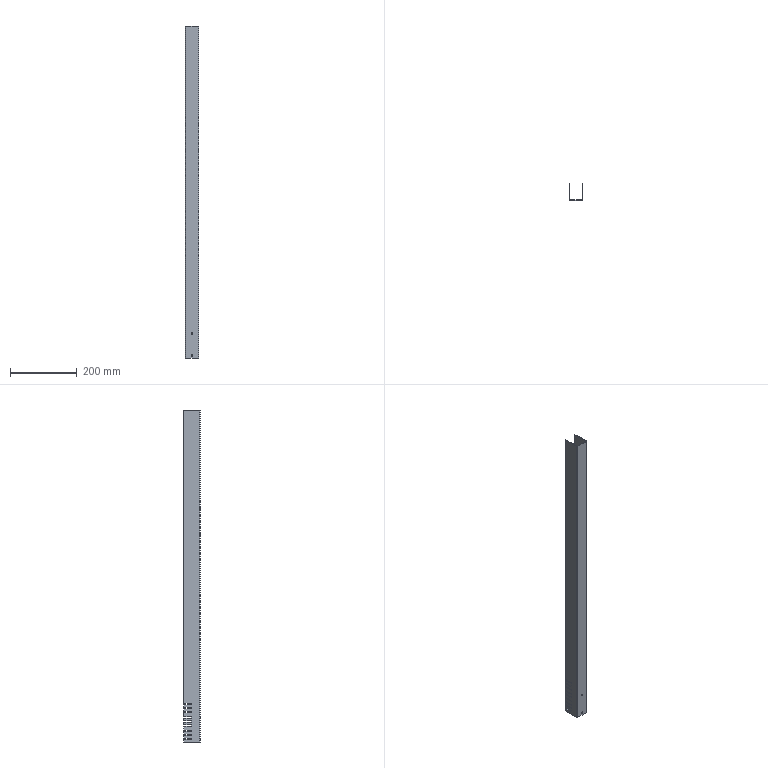Part | SolidWorks | features Cut 1, FlatPattern 1, ICE 1, LPattern 1, SMBaseFlange 1, SheetMetal 1 | 1 solid | 98 faces | box 40 x 50 x 996 mm | volume 200873 mm3 | plane 90 | cylinder 8 | commonest cylinder face diameters 5 x4 0.4 x2 3.4 x2